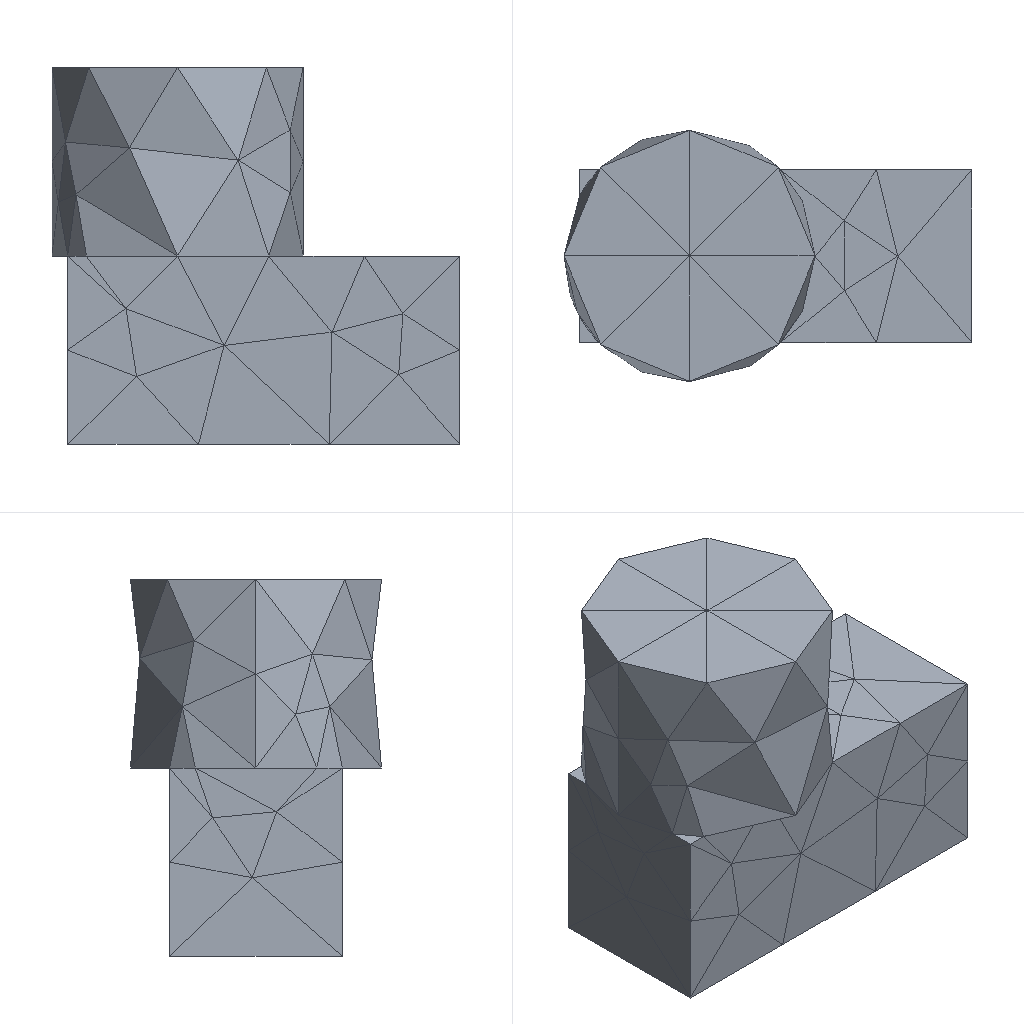Simulation study | ansys mapdl
Set-up summary:
category,name,step,type,value,unit,region
solver,ansys_mapdl
units,mm-N-s-tonne (MPa),,inferred,E=210000 density=
analysis,model,,static
mesh,nodes,,,483
mesh,elements,,,236
element_type,SOLID187,,,236
material,mat 1,,E,210000
material,mat 1,,nu,0.3
load,,model,body load temp,,,all
load,,model,force,"1000 [dir=(0, 0, -1) n=60]",,node list
bc,,model,fixed,"[dofs=UX,UY,UZ n=435]",,node list
Ansys APDL input file, long lists of numbers shortened:
/COM,ANSYS RELEASE 2026 R1           BUILD 26.1      UP20260202       09:10:51
/PREP7
/NOPR
/TITLE,2
ANTYPE, 0
*IF,_CDRDOFF,EQ,1,THEN     !if solid model was read in
_CDRDOFF=             !reset flag, numoffs already performed
*ELSE              !offset database for the following FE model
NUMOFF,NODE,      483
NUMOFF,ELEM,      236
NUMOFF,MAT ,        1
NUMOFF,TYPE,        1
*ENDIF
*SET,_RETURN ,  0.
*SET,_STATUS ,  0.
*SET,_UIQR   ,  60.
*SET,__FLOATPARAMETER__,  483.
DOF,DELETE
ETBLOCK,        1,        1
(2i9,19a9)
        1      187        0        0        0        0        0        0        0        0        0        0        0        0        0        0        0        0        0        0        0
       -1
NBLOCK,6,SOLID,       483,       483
(3i9,6e21.13e3)
        1        0        0 1.1000000000000E+001 1.1000000000000E+001 6.0000000000000E+001
! (482 more lines like these left out)
N,UNBL,LOC,       -1,
EBLOCK,19,SOLID,       236,       236
(19i10)
         1         1         1         1         0         0         0         0        10         0         1       299       254       216       199       310       311       312       313
! (471 more lines like these left out)
        -1
MPTEMP,UNBL, 1, 1,  0.    ,
MPDATA,UNBL, 1,EX  ,       1, 1,  210000.000    ,
MPTEMP,UNBL, 1, 1,  0.    ,
MPDATA,UNBL, 1,NUXY,       1, 1, 0.3    ,
MPTEMP,UNBL, 1, 1,  0.    ,
MPDATA,UNBL, 1,PRXY,       1, 1, 0.3    ,
EXTOPT,ATTR,      0,      0,      0
EXTOPT,ESIZE,  0,  0.
EXTOPT,ACLEAR,      0
TREF,  0.
IRLF,  0
BFUNIF,TEMP,_TINY
ACEL,  0.    ,  0.    ,  0.
OMEGA,  0.    ,  0.    ,  0.
DOMEGA,  0.    ,  0.    ,  0.
CGLOC,  0.    ,  0.    ,  0.
CGOMEGA,  0.    ,  0.    ,  0.
DCGOMG,  0.    ,  0.    ,  0.
KUSE,     0
TIME,  0.
ALPHAD,  0.
BETAD,  0.
DMPRAT,  0.
DMPSTR,  0.
CRPLIM, 0.1    ,   0
CRPLIM,  0.    ,   1
NCNV,     0, 1.000000000E+12,     0,  0.    ,  0.
NEQIT,     0
ERESX,DEFA
DBLOCK,       435
(i9,a6,2(pg16.9))
        1  UX    0.00000000      0.00000000
! (434 more lines like these left out)
       -1
FBLOCK,        60
(i9,a6,2(pg16.9))
      192  FZ   -16.6666667      0.00000000
! (59 more lines like these left out)
       -1
/GO
FINISH
Results summary:
result,analysis_type_db,,,static,unstated
result,n_sets,,,1,unstated
result,load_steps[0].set,load_step=1,,1,unstated
result,load_steps[0].substep,load_step=1,,1,unstated
result,load_steps[0].time,load_step=1,,1,unstated
result,load_steps[0].freq,load_step=1,,1,unstated
result,load_steps[0].max_usum,load_step=1,,0.000595,unstated
result,load_steps[0].max_seqv,load_step=1,,8.212,unstated
result,load_steps[0].reaction_sum.FX,load_step=1,,2.78035e-11,unstated
result,load_steps[0].reaction_sum.FY,load_step=1,,2.92744e-12,unstated
result,load_steps[0].reaction_sum.FZ,load_step=1,,1000,unstated
result,load_steps[0].reaction_sum.MX,load_step=1,,0,unstated
result,load_steps[0].reaction_sum.MY,load_step=1,,0,unstated
result,load_steps[0].reaction_sum.MZ,load_step=1,,0,unstated
result,convergence,,,results present for all listed sets,unstated